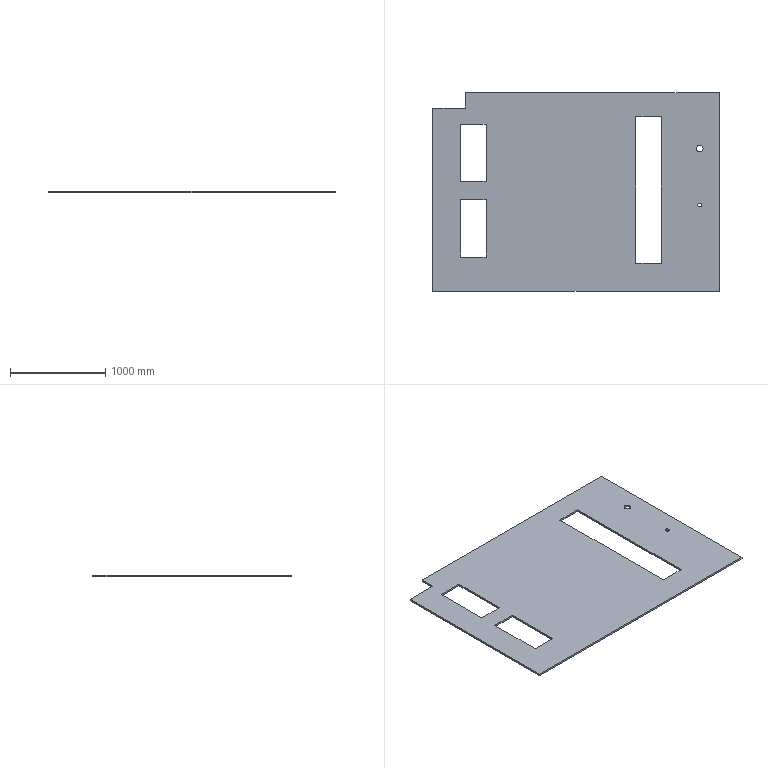Part | STEP file | 果蔬烘干机框架-104 | 1 solid | 24 faces | box 3000 x 2080 x 20 mm | volume 109217649 mm3 | plane 20 | cylinder 4 | commonest cylinder face diameters 40 x2 70 x2
STEP:
#1=CARTESIAN_POINT('',(1316.,-135.8,20.));
#2=VERTEX_POINT('',#1);
#3=CARTESIAN_POINT('',(1276.,-135.8,20.));
#4=VERTEX_POINT('',#3);
#5=CARTESIAN_POINT('',(1296.,-135.8,20.));
#6=DIRECTION('',(0.,0.,-1.));
#7=DIRECTION('',(-1.,0.,0.));
#8=AXIS2_PLACEMENT_3D('',#5,#6,#7);
#9=CIRCLE('',#8,20.);
#10=EDGE_CURVE('',#2,#4,#9,.T.);
#11=ORIENTED_EDGE('',*,*,#10,.F.);
#12=CARTESIAN_POINT('',(1316.,-135.8,0.));
#13=VERTEX_POINT('',#12);
#14=CARTESIAN_POINT('',(1316.,-135.8,20.));
#15=DIRECTION('',(0.,0.,-1.));
#16=VECTOR('',#15,1000.);
#17=LINE('',#14,#16);
#18=EDGE_CURVE('',#2,#13,#17,.T.);
#19=ORIENTED_EDGE('',*,*,#18,.T.);
#20=CARTESIAN_POINT('',(1276.,-135.8,0.));
#21=VERTEX_POINT('',#20);
#22=CARTESIAN_POINT('',(1296.,-135.8,0.));
#23=DIRECTION('',(0.,0.,-1.));
#24=DIRECTION('',(-1.,0.,0.));
#25=AXIS2_PLACEMENT_3D('',#22,#23,#24);
#26=CIRCLE('',#25,20.);
#27=EDGE_CURVE('',#13,#21,#26,.T.);
#28=ORIENTED_EDGE('',*,*,#27,.T.);
#29=CARTESIAN_POINT('',(1276.,-135.8,20.));
#30=DIRECTION('',(0.,0.,-1.));
#31=VECTOR('',#30,1000.);
#32=LINE('',#29,#31);
#33=EDGE_CURVE('',#4,#21,#32,.T.);
#34=ORIENTED_EDGE('',*,*,#33,.F.);
#35=EDGE_LOOP('',(#11,#19,#28,#34));
#36=FACE_OUTER_BOUND('',#35,.T.);
#37=CARTESIAN_POINT('',(1296.,-135.8,20.));
#38=DIRECTION('',(0.,0.,-1.));
#39=DIRECTION('',(-1.,0.,0.));
#40=AXIS2_PLACEMENT_3D('',#37,#38,#39);
#41=CYLINDRICAL_SURFACE('',#40,20.);
#42=ADVANCED_FACE('',(#36),#41,.F.);
#43=CARTESIAN_POINT('',(1331.,454.2,20.));
#44=VERTEX_POINT('',#43);
#45=CARTESIAN_POINT('',(1261.,454.2,20.));
#46=VERTEX_POINT('',#45);
#47=CARTESIAN_POINT('',(1296.,454.2,20.));
#48=DIRECTION('',(0.,0.,-1.));
#49=DIRECTION('',(-1.,0.,0.));
#50=AXIS2_PLACEMENT_3D('',#47,#48,#49);
#51=CIRCLE('',#50,35.);
#52=EDGE_CURVE('',#44,#46,#51,.T.);
#53=ORIENTED_EDGE('',*,*,#52,.F.);
#54=CARTESIAN_POINT('',(1331.,454.2,0.));
#55=VERTEX_POINT('',#54);
#56=CARTESIAN_POINT('',(1331.,454.2,20.));
#57=DIRECTION('',(0.,0.,-1.));
#58=VECTOR('',#57,1000.);
#59=LINE('',#56,#58);
#60=EDGE_CURVE('',#44,#55,#59,.T.);
#61=ORIENTED_EDGE('',*,*,#60,.T.);
#62=CARTESIAN_POINT('',(1261.,454.2,0.));
#63=VERTEX_POINT('',#62);
#64=CARTESIAN_POINT('',(1296.,454.2,0.));
#65=DIRECTION('',(0.,0.,-1.));
#66=DIRECTION('',(-1.,0.,0.));
#67=AXIS2_PLACEMENT_3D('',#64,#65,#66);
#68=CIRCLE('',#67,35.);
#69=EDGE_CURVE('',#55,#63,#68,.T.);
#70=ORIENTED_EDGE('',*,*,#69,.T.);
#71=CARTESIAN_POINT('',(1261.,454.2,20.));
#72=DIRECTION('',(0.,0.,-1.));
#73=VECTOR('',#72,1000.);
#74=LINE('',#71,#73);
#75=EDGE_CURVE('',#46,#63,#74,.T.);
#76=ORIENTED_EDGE('',*,*,#75,.F.);
#77=EDGE_LOOP('',(#53,#61,#70,#76));
#78=FACE_OUTER_BOUND('',#77,.T.);
#79=CARTESIAN_POINT('',(1296.,454.2,20.));
#80=DIRECTION('',(0.,0.,-1.));
#81=DIRECTION('',(-1.,0.,0.));
#82=AXIS2_PLACEMENT_3D('',#79,#80,#81);
#83=CYLINDRICAL_SURFACE('',#82,35.);
#84=ADVANCED_FACE('',(#78),#83,.F.);
#85=CARTESIAN_POINT('',(-1500.,880.,0.));
#86=VERTEX_POINT('',#85);
#87=CARTESIAN_POINT('',(-1500.,880.,20.));
#88=VERTEX_POINT('',#87);
#89=CARTESIAN_POINT('',(-1500.,880.,-80.));
#90=DIRECTION('',(0.,0.,1.));
#91=VECTOR('',#90,1000.);
#92=LINE('',#89,#91);
#93=EDGE_CURVE('',#86,#88,#92,.T.);
#94=ORIENTED_EDGE('',*,*,#93,.F.);
#95=CARTESIAN_POINT('',(-1500.,-1040.,0.));
#96=VERTEX_POINT('',#95);
#97=CARTESIAN_POINT('',(-1500.,1040.,0.));
#98=DIRECTION('',(0.,-1.,0.));
#99=VECTOR('',#98,1000.);
#100=LINE('',#97,#99);
#101=EDGE_CURVE('',#86,#96,#100,.T.);
#102=ORIENTED_EDGE('',*,*,#101,.T.);
#103=CARTESIAN_POINT('',(-1500.,-1040.,20.));
#104=VERTEX_POINT('',#103);
#105=CARTESIAN_POINT('',(-1500.,-1040.,20.));
#106=DIRECTION('',(0.,0.,-1.));
#107=VECTOR('',#106,1000.);
#108=LINE('',#105,#107);
#109=EDGE_CURVE('',#104,#96,#108,.T.);
#110=ORIENTED_EDGE('',*,*,#109,.F.);
#111=CARTESIAN_POINT('',(-1500.,1040.,20.));
#112=DIRECTION('',(0.,-1.,0.));
#113=VECTOR('',#112,1000.);
#114=LINE('',#111,#113);
#115=EDGE_CURVE('',#88,#104,#114,.T.);
#116=ORIENTED_EDGE('',*,*,#115,.F.);
#117=EDGE_LOOP('',(#94,#102,#110,#116));
#118=FACE_OUTER_BOUND('',#117,.T.);
#119=CARTESIAN_POINT('',(-1500.,1040.,20.));
#120=DIRECTION('',(1.,0.,0.));
#121=DIRECTION('',(0.,1.,0.));
#122=AXIS2_PLACEMENT_3D('',#119,#120,#121);
#123=PLANE('',#122);
#124=ADVANCED_FACE('',(#118),#123,.F.);
#125=CARTESIAN_POINT('',(1500.,-1040.,0.));
#126=VERTEX_POINT('',#125);
#127=CARTESIAN_POINT('',(1500.,1040.,0.));
#128=VERTEX_POINT('',#127);
#129=CARTESIAN_POINT('',(1500.,1040.,0.));
#130=DIRECTION('',(0.,1.,0.));
#131=VECTOR('',#130,1000.);
#132=LINE('',#129,#131);
#133=EDGE_CURVE('',#126,#128,#132,.T.);
#134=ORIENTED_EDGE('',*,*,#133,.T.);
#135=CARTESIAN_POINT('',(1500.,1040.,20.));
#136=VERTEX_POINT('',#135);
#137=CARTESIAN_POINT('',(1500.,1040.,20.));
#138=DIRECTION('',(0.,0.,-1.));
#139=VECTOR('',#138,1000.);
#140=LINE('',#137,#139);
#141=EDGE_CURVE('',#136,#128,#140,.T.);
#142=ORIENTED_EDGE('',*,*,#141,.F.);
#143=CARTESIAN_POINT('',(1500.,-1040.,20.));
#144=VERTEX_POINT('',#143);
#145=CARTESIAN_POINT('',(1500.,1040.,20.));
#146=DIRECTION('',(0.,1.,0.));
#147=VECTOR('',#146,1000.);
#148=LINE('',#145,#147);
#149=EDGE_CURVE('',#144,#136,#148,.T.);
#150=ORIENTED_EDGE('',*,*,#149,.F.);
#151=CARTESIAN_POINT('',(1500.,-1040.,20.));
#152=DIRECTION('',(0.,0.,-1.));
#153=VECTOR('',#152,1000.);
#154=LINE('',#151,#153);
#155=EDGE_CURVE('',#144,#126,#154,.T.);
#156=ORIENTED_EDGE('',*,*,#155,.T.);
#157=EDGE_LOOP('',(#134,#142,#150,#156));
#158=FACE_OUTER_BOUND('',#157,.T.);
#159=CARTESIAN_POINT('',(1500.,1040.,20.));
#160=DIRECTION('',(-1.,0.,0.));
#161=DIRECTION('',(0.,-1.,0.));
#162=AXIS2_PLACEMENT_3D('',#159,#160,#161);
#163=PLANE('',#162);
#164=ADVANCED_FACE('',(#158),#163,.F.);
#165=CARTESIAN_POINT('',(-1160.,1040.,0.));
#166=VERTEX_POINT('',#165);
#167=CARTESIAN_POINT('',(-1500.,1040.,0.));
#168=DIRECTION('',(-1.,0.,0.));
#169=VECTOR('',#168,1000.);
#170=LINE('',#167,#169);
#171=EDGE_CURVE('',#128,#166,#170,.T.);
#172=ORIENTED_EDGE('',*,*,#171,.T.);
#173=CARTESIAN_POINT('',(-1160.,1040.,20.));
#174=VERTEX_POINT('',#173);
#175=CARTESIAN_POINT('',(-1160.,1040.,-80.));
#176=DIRECTION('',(0.,0.,1.));
#177=VECTOR('',#176,1000.);
#178=LINE('',#175,#177);
#179=EDGE_CURVE('',#166,#174,#178,.T.);
#180=ORIENTED_EDGE('',*,*,#179,.T.);
#181=CARTESIAN_POINT('',(-1500.,1040.,20.));
#182=DIRECTION('',(-1.,0.,0.));
#183=VECTOR('',#182,1000.);
#184=LINE('',#181,#183);
#185=EDGE_CURVE('',#136,#174,#184,.T.);
#186=ORIENTED_EDGE('',*,*,#185,.F.);
#187=ORIENTED_EDGE('',*,*,#141,.T.);
#188=EDGE_LOOP('',(#172,#180,#186,#187));
#189=FACE_OUTER_BOUND('',#188,.T.);
#190=CARTESIAN_POINT('',(-1500.,1040.,20.));
#191=DIRECTION('',(0.,-1.,0.));
#192=DIRECTION('',(0.,0.,-1.));
#193=AXIS2_PLACEMENT_3D('',#190,#191,#192);
#194=PLANE('',#193);
#195=ADVANCED_FACE('',(#189),#194,.F.);
#196=CARTESIAN_POINT('',(-1500.,-1040.,0.));
#197=DIRECTION('',(1.,0.,0.));
#198=VECTOR('',#197,1000.);
#199=LINE('',#196,#198);
#200=EDGE_CURVE('',#96,#126,#199,.T.);
#201=ORIENTED_EDGE('',*,*,#200,.T.);
#202=ORIENTED_EDGE('',*,*,#155,.F.);
#203=CARTESIAN_POINT('',(-1500.,-1040.,20.));
#204=DIRECTION('',(1.,0.,0.));
#205=VECTOR('',#204,1000.);
#206=LINE('',#203,#205);
#207=EDGE_CURVE('',#104,#144,#206,.T.);
#208=ORIENTED_EDGE('',*,*,#207,.F.);
#209=ORIENTED_EDGE('',*,*,#109,.T.);
#210=EDGE_LOOP('',(#201,#202,#208,#209));
#211=FACE_OUTER_BOUND('',#210,.T.);
#212=CARTESIAN_POINT('',(-1500.,-1040.,20.));
#213=DIRECTION('',(0.,1.,0.));
#214=DIRECTION('',(0.,0.,1.));
#215=AXIS2_PLACEMENT_3D('',#212,#213,#214);
#216=PLANE('',#215);
#217=ADVANCED_FACE('',(#211),#216,.F.);
#218=CARTESIAN_POINT('',(1296.,-135.8,20.));
#219=DIRECTION('',(0.,0.,-1.));
#220=DIRECTION('',(-1.,0.,0.));
#221=AXIS2_PLACEMENT_3D('',#218,#219,#220);
#222=CIRCLE('',#221,20.);
#223=EDGE_CURVE('',#4,#2,#222,.T.);
#224=ORIENTED_EDGE('',*,*,#223,.T.);
#225=ORIENTED_EDGE('',*,*,#10,.T.);
#226=EDGE_LOOP('',(#224,#225));
#227=FACE_BOUND('',#226,.T.);
#228=CARTESIAN_POINT('',(1296.,454.2,20.));
#229=DIRECTION('',(0.,0.,-1.));
#230=DIRECTION('',(-1.,0.,0.));
#231=AXIS2_PLACEMENT_3D('',#228,#229,#230);
#232=CIRCLE('',#231,35.);
#233=EDGE_CURVE('',#46,#44,#232,.T.);
#234=ORIENTED_EDGE('',*,*,#233,.T.);
#235=ORIENTED_EDGE('',*,*,#52,.T.);
#236=EDGE_LOOP('',(#234,#235));
#237=FACE_BOUND('',#236,.T.);
#238=CARTESIAN_POINT('',(-943.,-81.276,20.));
#239=VERTEX_POINT('',#238);
#240=CARTESIAN_POINT('',(-943.,-681.324,20.));
#241=VERTEX_POINT('',#240);
#242=CARTESIAN_POINT('',(-943.,-81.276,20.));
#243=DIRECTION('',(0.,-1.,0.));
#244=VECTOR('',#243,1000.);
#245=LINE('',#242,#244);
#246=EDGE_CURVE('',#239,#241,#245,.T.);
#247=ORIENTED_EDGE('',*,*,#246,.T.);
#248=CARTESIAN_POINT('',(-1206.,-681.324,20.));
#249=VERTEX_POINT('',#248);
#250=CARTESIAN_POINT('',(-943.,-681.324,20.));
#251=DIRECTION('',(-1.,0.,0.));
#252=VECTOR('',#251,1000.);
#253=LINE('',#250,#252);
#254=EDGE_CURVE('',#241,#249,#253,.T.);
#255=ORIENTED_EDGE('',*,*,#254,.T.);
#256=CARTESIAN_POINT('',(-1206.,-81.276,20.));
#257=VERTEX_POINT('',#256);
#258=CARTESIAN_POINT('',(-1206.,-81.276,20.));
#259=DIRECTION('',(0.,1.,0.));
#260=VECTOR('',#259,1000.);
#261=LINE('',#258,#260);
#262=EDGE_CURVE('',#249,#257,#261,.T.);
#263=ORIENTED_EDGE('',*,*,#262,.T.);
#264=CARTESIAN_POINT('',(-943.,-81.276,20.));
#265=DIRECTION('',(1.,0.,0.));
#266=VECTOR('',#265,1000.);
#267=LINE('',#264,#266);
#268=EDGE_CURVE('',#257,#239,#267,.T.);
#269=ORIENTED_EDGE('',*,*,#268,.T.);
#270=EDGE_LOOP('',(#247,#255,#263,#269));
#271=FACE_BOUND('',#270,.T.);
#272=CARTESIAN_POINT('',(-943.,711.724,20.));
#273=VERTEX_POINT('',#272);
#274=CARTESIAN_POINT('',(-943.,111.676,20.));
#275=VERTEX_POINT('',#274);
#276=CARTESIAN_POINT('',(-943.,711.724,20.));
#277=DIRECTION('',(0.,-1.,0.));
#278=VECTOR('',#277,1000.);
#279=LINE('',#276,#278);
#280=EDGE_CURVE('',#273,#275,#279,.T.);
#281=ORIENTED_EDGE('',*,*,#280,.T.);
#282=CARTESIAN_POINT('',(-1206.,111.676,20.));
#283=VERTEX_POINT('',#282);
#284=CARTESIAN_POINT('',(-943.,111.676,20.));
#285=DIRECTION('',(-1.,0.,0.));
#286=VECTOR('',#285,1000.);
#287=LINE('',#284,#286);
#288=EDGE_CURVE('',#275,#283,#287,.T.);
#289=ORIENTED_EDGE('',*,*,#288,.T.);
#290=CARTESIAN_POINT('',(-1206.,711.724,20.));
#291=VERTEX_POINT('',#290);
#292=CARTESIAN_POINT('',(-1206.,711.724,20.));
#293=DIRECTION('',(0.,1.,0.));
#294=VECTOR('',#293,1000.);
#295=LINE('',#292,#294);
#296=EDGE_CURVE('',#283,#291,#295,.T.);
#297=ORIENTED_EDGE('',*,*,#296,.T.);
#298=CARTESIAN_POINT('',(-943.,711.724,20.));
#299=DIRECTION('',(1.,0.,0.));
#300=VECTOR('',#299,1000.);
#301=LINE('',#298,#300);
#302=EDGE_CURVE('',#291,#273,#301,.T.);
#303=ORIENTED_EDGE('',*,*,#302,.T.);
#304=EDGE_LOOP('',(#281,#289,#297,#303));
#305=FACE_BOUND('',#304,.T.);
#306=CARTESIAN_POINT('',(891.55,788.541,20.));
#307=VERTEX_POINT('',#306);
#308=CARTESIAN_POINT('',(891.55,-746.951,20.));
#309=VERTEX_POINT('',#308);
#310=CARTESIAN_POINT('',(891.55,788.541,20.));
#311=DIRECTION('',(0.,-1.,0.));
#312=VECTOR('',#311,1000.);
#313=LINE('',#310,#312);
#314=EDGE_CURVE('',#307,#309,#313,.T.);
#315=ORIENTED_EDGE('',*,*,#314,.T.);
#316=CARTESIAN_POINT('',(628.45,-746.951,20.));
#317=VERTEX_POINT('',#316);
#318=CARTESIAN_POINT('',(891.55,-746.951,20.));
#319=DIRECTION('',(-1.,0.,0.));
#320=VECTOR('',#319,1000.);
#321=LINE('',#318,#320);
#322=EDGE_CURVE('',#309,#317,#321,.T.);
#323=ORIENTED_EDGE('',*,*,#322,.T.);
#324=CARTESIAN_POINT('',(628.45,788.541,20.));
#325=VERTEX_POINT('',#324);
#326=CARTESIAN_POINT('',(628.45,788.541,20.));
#327=DIRECTION('',(0.,1.,0.));
#328=VECTOR('',#327,1000.);
#329=LINE('',#326,#328);
#330=EDGE_CURVE('',#317,#325,#329,.T.);
#331=ORIENTED_EDGE('',*,*,#330,.T.);
#332=CARTESIAN_POINT('',(891.55,788.541,20.));
#333=DIRECTION('',(1.,0.,0.));
#334=VECTOR('',#333,1000.);
#335=LINE('',#332,#334);
#336=EDGE_CURVE('',#325,#307,#335,.T.);
#337=ORIENTED_EDGE('',*,*,#336,.T.);
#338=EDGE_LOOP('',(#315,#323,#331,#337));
#339=FACE_BOUND('',#338,.T.);
#340=CARTESIAN_POINT('',(-1160.,880.,20.));
#341=VERTEX_POINT('',#340);
#342=CARTESIAN_POINT('',(-1500.,880.,20.));
#343=DIRECTION('',(1.,0.,0.));
#344=VECTOR('',#343,1000.);
#345=LINE('',#342,#344);
#346=EDGE_CURVE('',#88,#341,#345,.T.);
#347=ORIENTED_EDGE('',*,*,#346,.F.);
#348=ORIENTED_EDGE('',*,*,#115,.T.);
#349=ORIENTED_EDGE('',*,*,#207,.T.);
#350=ORIENTED_EDGE('',*,*,#149,.T.);
#351=ORIENTED_EDGE('',*,*,#185,.T.);
#352=CARTESIAN_POINT('',(-1160.,1040.,20.));
#353=DIRECTION('',(0.,1.,0.));
#354=VECTOR('',#353,1000.);
#355=LINE('',#352,#354);
#356=EDGE_CURVE('',#341,#174,#355,.T.);
#357=ORIENTED_EDGE('',*,*,#356,.F.);
#358=EDGE_LOOP('',(#347,#348,#349,#350,#351,#357));
#359=FACE_OUTER_BOUND('',#358,.T.);
#360=CARTESIAN_POINT('',(0.,0.,20.));
#361=DIRECTION('',(0.,0.,1.));
#362=DIRECTION('',(1.,0.,0.));
#363=AXIS2_PLACEMENT_3D('',#360,#361,#362);
#364=PLANE('',#363);
#365=ADVANCED_FACE('',(#227,#237,#271,#305,#339,#359),#364,.T.);
#366=CARTESIAN_POINT('',(1296.,-135.8,0.));
#367=DIRECTION('',(0.,0.,-1.));
#368=DIRECTION('',(-1.,0.,0.));
#369=AXIS2_PLACEMENT_3D('',#366,#367,#368);
#370=CIRCLE('',#369,20.);
#371=EDGE_CURVE('',#21,#13,#370,.T.);
#372=ORIENTED_EDGE('',*,*,#371,.F.);
#373=ORIENTED_EDGE('',*,*,#27,.F.);
#374=EDGE_LOOP('',(#372,#373));
#375=FACE_BOUND('',#374,.T.);
#376=CARTESIAN_POINT('',(1296.,454.2,0.));
#377=DIRECTION('',(0.,0.,-1.));
#378=DIRECTION('',(-1.,0.,0.));
#379=AXIS2_PLACEMENT_3D('',#376,#377,#378);
#380=CIRCLE('',#379,35.);
#381=EDGE_CURVE('',#63,#55,#380,.T.);
#382=ORIENTED_EDGE('',*,*,#381,.F.);
#383=ORIENTED_EDGE('',*,*,#69,.F.);
#384=EDGE_LOOP('',(#382,#383));
#385=FACE_BOUND('',#384,.T.);
#386=CARTESIAN_POINT('',(-943.,-681.324,0.));
#387=VERTEX_POINT('',#386);
#388=CARTESIAN_POINT('',(-1206.,-681.324,0.));
#389=VERTEX_POINT('',#388);
#390=CARTESIAN_POINT('',(-943.,-681.324,0.));
#391=DIRECTION('',(-1.,0.,0.));
#392=VECTOR('',#391,1000.);
#393=LINE('',#390,#392);
#394=EDGE_CURVE('',#387,#389,#393,.T.);
#395=ORIENTED_EDGE('',*,*,#394,.F.);
#396=CARTESIAN_POINT('',(-943.,-81.276,0.));
#397=VERTEX_POINT('',#396);
#398=CARTESIAN_POINT('',(-943.,-81.276,0.));
#399=DIRECTION('',(0.,-1.,0.));
#400=VECTOR('',#399,1000.);
#401=LINE('',#398,#400);
#402=EDGE_CURVE('',#397,#387,#401,.T.);
#403=ORIENTED_EDGE('',*,*,#402,.F.);
#404=CARTESIAN_POINT('',(-1206.,-81.276,0.));
#405=VERTEX_POINT('',#404);
#406=CARTESIAN_POINT('',(-943.,-81.276,0.));
#407=DIRECTION('',(1.,0.,0.));
#408=VECTOR('',#407,1000.);
#409=LINE('',#406,#408);
#410=EDGE_CURVE('',#405,#397,#409,.T.);
#411=ORIENTED_EDGE('',*,*,#410,.F.);
#412=CARTESIAN_POINT('',(-1206.,-81.276,0.));
#413=DIRECTION('',(0.,1.,0.));
#414=VECTOR('',#413,1000.);
#415=LINE('',#412,#414);
#416=EDGE_CURVE('',#389,#405,#415,.T.);
#417=ORIENTED_EDGE('',*,*,#416,.F.);
#418=EDGE_LOOP('',(#395,#403,#411,#417));
#419=FACE_BOUND('',#418,.T.);
#420=CARTESIAN_POINT('',(-943.,111.676,0.));
#421=VERTEX_POINT('',#420);
#422=CARTESIAN_POINT('',(-1206.,111.676,0.));
#423=VERTEX_POINT('',#422);
#424=CARTESIAN_POINT('',(-943.,111.676,0.));
#425=DIRECTION('',(-1.,0.,0.));
#426=VECTOR('',#425,1000.);
#427=LINE('',#424,#426);
#428=EDGE_CURVE('',#421,#423,#427,.T.);
#429=ORIENTED_EDGE('',*,*,#428,.F.);
#430=CARTESIAN_POINT('',(-943.,711.724,0.));
#431=VERTEX_POINT('',#430);
#432=CARTESIAN_POINT('',(-943.,711.724,0.));
#433=DIRECTION('',(0.,-1.,0.));
#434=VECTOR('',#433,1000.);
#435=LINE('',#432,#434);
#436=EDGE_CURVE('',#431,#421,#435,.T.);
#437=ORIENTED_EDGE('',*,*,#436,.F.);
#438=CARTESIAN_POINT('',(-1206.,711.724,0.));
#439=VERTEX_POINT('',#438);
#440=CARTESIAN_POINT('',(-943.,711.724,0.));
#441=DIRECTION('',(1.,0.,0.));
#442=VECTOR('',#441,1000.);
#443=LINE('',#440,#442);
#444=EDGE_CURVE('',#439,#431,#443,.T.);
#445=ORIENTED_EDGE('',*,*,#444,.F.);
#446=CARTESIAN_POINT('',(-1206.,711.724,0.));
#447=DIRECTION('',(0.,1.,0.));
#448=VECTOR('',#447,1000.);
#449=LINE('',#446,#448);
#450=EDGE_CURVE('',#423,#439,#449,.T.);
#451=ORIENTED_EDGE('',*,*,#450,.F.);
#452=EDGE_LOOP('',(#429,#437,#445,#451));
#453=FACE_BOUND('',#452,.T.);
#454=CARTESIAN_POINT('',(891.55,-746.951,0.));
#455=VERTEX_POINT('',#454);
#456=CARTESIAN_POINT('',(628.45,-746.951,0.));
#457=VERTEX_POINT('',#456);
#458=CARTESIAN_POINT('',(891.55,-746.951,0.));
#459=DIRECTION('',(-1.,0.,0.));
#460=VECTOR('',#459,1000.);
#461=LINE('',#458,#460);
#462=EDGE_CURVE('',#455,#457,#461,.T.);
#463=ORIENTED_EDGE('',*,*,#462,.F.);
#464=CARTESIAN_POINT('',(891.55,788.541,0.));
#465=VERTEX_POINT('',#464);
#466=CARTESIAN_POINT('',(891.55,788.541,0.));
#467=DIRECTION('',(0.,-1.,0.));
#468=VECTOR('',#467,1000.);
#469=LINE('',#466,#468);
#470=EDGE_CURVE('',#465,#455,#469,.T.);
#471=ORIENTED_EDGE('',*,*,#470,.F.);
#472=CARTESIAN_POINT('',(628.45,788.541,0.));
#473=VERTEX_POINT('',#472);
#474=CARTESIAN_POINT('',(891.55,788.541,0.));
#475=DIRECTION('',(1.,0.,0.));
#476=VECTOR('',#475,1000.);
#477=LINE('',#474,#476);
#478=EDGE_CURVE('',#473,#465,#477,.T.);
#479=ORIENTED_EDGE('',*,*,#478,.F.);
#480=CARTESIAN_POINT('',(628.45,788.541,0.));
#481=DIRECTION('',(0.,1.,0.));
#482=VECTOR('',#481,1000.);
#483=LINE('',#480,#482);
#484=EDGE_CURVE('',#457,#473,#483,.T.);
#485=ORIENTED_EDGE('',*,*,#484,.F.);
#486=EDGE_LOOP('',(#463,#471,#479,#485));
#487=FACE_BOUND('',#486,.T.);
#488=CARTESIAN_POINT('',(-1160.,880.,0.));
#489=VERTEX_POINT('',#488);
#490=CARTESIAN_POINT('',(0.,880.,0.));
#491=DIRECTION('',(1.,0.,0.));
#492=VECTOR('',#491,1000.);
#493=LINE('',#490,#492);
#494=EDGE_CURVE('',#86,#489,#493,.T.);
#495=ORIENTED_EDGE('',*,*,#494,.T.);
#496=CARTESIAN_POINT('',(-1160.,0.,0.));
#497=DIRECTION('',(0.,1.,0.));
#498=VECTOR('',#497,1000.);
#499=LINE('',#496,#498);
#500=EDGE_CURVE('',#489,#166,#499,.T.);
#501=ORIENTED_EDGE('',*,*,#500,.T.);
#502=ORIENTED_EDGE('',*,*,#171,.F.);
#503=ORIENTED_EDGE('',*,*,#133,.F.);
#504=ORIENTED_EDGE('',*,*,#200,.F.);
#505=ORIENTED_EDGE('',*,*,#101,.F.);
#506=EDGE_LOOP('',(#495,#501,#502,#503,#504,#505));
#507=FACE_OUTER_BOUND('',#506,.T.);
#508=CARTESIAN_POINT('',(0.,0.,0.));
#509=DIRECTION('',(0.,0.,1.));
#510=DIRECTION('',(1.,0.,0.));
#511=AXIS2_PLACEMENT_3D('',#508,#509,#510);
#512=PLANE('',#511);
#513=ADVANCED_FACE('',(#375,#385,#419,#453,#487,#507),#512,.F.);
#514=CARTESIAN_POINT('',(-1160.,880.,-80.));
#515=DIRECTION('',(0.,0.,1.));
#516=VECTOR('',#515,1000.);
#517=LINE('',#514,#516);
#518=EDGE_CURVE('',#489,#341,#517,.T.);
#519=ORIENTED_EDGE('',*,*,#518,.T.);
#520=ORIENTED_EDGE('',*,*,#356,.T.);
#521=ORIENTED_EDGE('',*,*,#179,.F.);
#522=ORIENTED_EDGE('',*,*,#500,.F.);
#523=EDGE_LOOP('',(#519,#520,#521,#522));
#524=FACE_OUTER_BOUND('',#523,.T.);
#525=CARTESIAN_POINT('',(-1160.,1040.,-80.));
#526=DIRECTION('',(1.,0.,0.));
#527=DIRECTION('',(0.,0.,-1.));
#528=AXIS2_PLACEMENT_3D('',#525,#526,#527);
#529=PLANE('',#528);
#530=ADVANCED_FACE('',(#524),#529,.F.);
#531=ORIENTED_EDGE('',*,*,#93,.T.);
#532=ORIENTED_EDGE('',*,*,#346,.T.);
#533=ORIENTED_EDGE('',*,*,#518,.F.);
#534=ORIENTED_EDGE('',*,*,#494,.F.);
#535=EDGE_LOOP('',(#531,#532,#533,#534));
#536=FACE_OUTER_BOUND('',#535,.T.);
#537=CARTESIAN_POINT('',(-1500.,880.,-80.));
#538=DIRECTION('',(0.,-1.,0.));
#539=DIRECTION('',(0.,0.,-1.));
#540=AXIS2_PLACEMENT_3D('',#537,#538,#539);
#541=PLANE('',#540);
#542=ADVANCED_FACE('',(#536),#541,.F.);
#543=ORIENTED_EDGE('',*,*,#470,.T.);
#544=CARTESIAN_POINT('',(891.55,-746.951,20.));
#545=DIRECTION('',(0.,0.,-1.));
#546=VECTOR('',#545,1000.);
#547=LINE('',#544,#546);
#548=EDGE_CURVE('',#309,#455,#547,.T.);
#549=ORIENTED_EDGE('',*,*,#548,.F.);
#550=ORIENTED_EDGE('',*,*,#314,.F.);
#551=CARTESIAN_POINT('',(891.55,788.541,20.));
#552=DIRECTION('',(0.,0.,-1.));
#553=VECTOR('',#552,1000.);
#554=LINE('',#551,#553);
#555=EDGE_CURVE('',#307,#465,#554,.T.);
#556=ORIENTED_EDGE('',*,*,#555,.T.);
#557=EDGE_LOOP('',(#543,#549,#550,#556));
#558=FACE_OUTER_BOUND('',#557,.T.);
#559=CARTESIAN_POINT('',(891.55,788.541,20.));
#560=DIRECTION('',(1.,0.,0.));
#561=DIRECTION('',(0.,1.,0.));
#562=AXIS2_PLACEMENT_3D('',#559,#560,#561);
#563=PLANE('',#562);
#564=ADVANCED_FACE('',(#558),#563,.F.);
#565=ORIENTED_EDGE('',*,*,#478,.T.);
#566=ORIENTED_EDGE('',*,*,#555,.F.);
#567=ORIENTED_EDGE('',*,*,#336,.F.);
#568=CARTESIAN_POINT('',(628.45,788.541,20.));
#569=DIRECTION('',(0.,0.,-1.));
#570=VECTOR('',#569,1000.);
#571=LINE('',#568,#570);
#572=EDGE_CURVE('',#325,#473,#571,.T.);
#573=ORIENTED_EDGE('',*,*,#572,.T.);
#574=EDGE_LOOP('',(#565,#566,#567,#573));
#575=FACE_OUTER_BOUND('',#574,.T.);
#576=CARTESIAN_POINT('',(891.55,788.541,20.));
#577=DIRECTION('',(0.,1.,0.));
#578=DIRECTION('',(0.,0.,1.));
#579=AXIS2_PLACEMENT_3D('',#576,#577,#578);
#580=PLANE('',#579);
#581=ADVANCED_FACE('',(#575),#580,.F.);
#582=ORIENTED_EDGE('',*,*,#484,.T.);
#583=ORIENTED_EDGE('',*,*,#572,.F.);
#584=ORIENTED_EDGE('',*,*,#330,.F.);
#585=CARTESIAN_POINT('',(628.45,-746.951,20.));
#586=DIRECTION('',(0.,0.,-1.));
#587=VECTOR('',#586,1000.);
#588=LINE('',#585,#587);
#589=EDGE_CURVE('',#317,#457,#588,.T.);
#590=ORIENTED_EDGE('',*,*,#589,.T.);
#591=EDGE_LOOP('',(#582,#583,#584,#590));
#592=FACE_OUTER_BOUND('',#591,.T.);
#593=CARTESIAN_POINT('',(628.45,788.541,20.));
#594=DIRECTION('',(-1.,0.,0.));
#595=DIRECTION('',(0.,-1.,0.));
#596=AXIS2_PLACEMENT_3D('',#593,#594,#595);
#597=PLANE('',#596);
#598=ADVANCED_FACE('',(#592),#597,.F.);
#599=ORIENTED_EDGE('',*,*,#462,.T.);
#600=ORIENTED_EDGE('',*,*,#589,.F.);
#601=ORIENTED_EDGE('',*,*,#322,.F.);
#602=ORIENTED_EDGE('',*,*,#548,.T.);
#603=EDGE_LOOP('',(#599,#600,#601,#602));
#604=FACE_OUTER_BOUND('',#603,.T.);
#605=CARTESIAN_POINT('',(891.55,-746.951,20.));
#606=DIRECTION('',(0.,-1.,0.));
#607=DIRECTION('',(0.,0.,-1.));
#608=AXIS2_PLACEMENT_3D('',#605,#606,#607);
#609=PLANE('',#608);
#610=ADVANCED_FACE('',(#604),#609,.F.);
#611=ORIENTED_EDGE('',*,*,#436,.T.);
#612=CARTESIAN_POINT('',(-943.,111.676,20.));
#613=DIRECTION('',(0.,0.,-1.));
#614=VECTOR('',#613,1000.);
#615=LINE('',#612,#614);
#616=EDGE_CURVE('',#275,#421,#615,.T.);
#617=ORIENTED_EDGE('',*,*,#616,.F.);
#618=ORIENTED_EDGE('',*,*,#280,.F.);
#619=CARTESIAN_POINT('',(-943.,711.724,20.));
#620=DIRECTION('',(0.,0.,-1.));
#621=VECTOR('',#620,1000.);
#622=LINE('',#619,#621);
#623=EDGE_CURVE('',#273,#431,#622,.T.);
#624=ORIENTED_EDGE('',*,*,#623,.T.);
#625=EDGE_LOOP('',(#611,#617,#618,#624));
#626=FACE_OUTER_BOUND('',#625,.T.);
#627=CARTESIAN_POINT('',(-943.,711.724,20.));
#628=DIRECTION('',(1.,0.,0.));
#629=DIRECTION('',(0.,1.,0.));
#630=AXIS2_PLACEMENT_3D('',#627,#628,#629);
#631=PLANE('',#630);
#632=ADVANCED_FACE('',(#626),#631,.F.);
#633=ORIENTED_EDGE('',*,*,#444,.T.);
#634=ORIENTED_EDGE('',*,*,#623,.F.);
#635=ORIENTED_EDGE('',*,*,#302,.F.);
#636=CARTESIAN_POINT('',(-1206.,711.724,20.));
#637=DIRECTION('',(0.,0.,-1.));
#638=VECTOR('',#637,1000.);
#639=LINE('',#636,#638);
#640=EDGE_CURVE('',#291,#439,#639,.T.);
#641=ORIENTED_EDGE('',*,*,#640,.T.);
#642=EDGE_LOOP('',(#633,#634,#635,#641));
#643=FACE_OUTER_BOUND('',#642,.T.);
#644=CARTESIAN_POINT('',(-943.,711.724,20.));
#645=DIRECTION('',(0.,1.,0.));
#646=DIRECTION('',(0.,0.,1.));
#647=AXIS2_PLACEMENT_3D('',#644,#645,#646);
#648=PLANE('',#647);
#649=ADVANCED_FACE('',(#643),#648,.F.);
#650=ORIENTED_EDGE('',*,*,#450,.T.);
#651=ORIENTED_EDGE('',*,*,#640,.F.);
#652=ORIENTED_EDGE('',*,*,#296,.F.);
#653=CARTESIAN_POINT('',(-1206.,111.676,20.));
#654=DIRECTION('',(0.,0.,-1.));
#655=VECTOR('',#654,1000.);
#656=LINE('',#653,#655);
#657=EDGE_CURVE('',#283,#423,#656,.T.);
#658=ORIENTED_EDGE('',*,*,#657,.T.);
#659=EDGE_LOOP('',(#650,#651,#652,#658));
#660=FACE_OUTER_BOUND('',#659,.T.);
#661=CARTESIAN_POINT('',(-1206.,711.724,20.));
#662=DIRECTION('',(-1.,0.,0.));
#663=DIRECTION('',(0.,0.,1.));
#664=AXIS2_PLACEMENT_3D('',#661,#662,#663);
#665=PLANE('',#664);
#666=ADVANCED_FACE('',(#660),#665,.F.);
#667=ORIENTED_EDGE('',*,*,#428,.T.);
#668=ORIENTED_EDGE('',*,*,#657,.F.);
#669=ORIENTED_EDGE('',*,*,#288,.F.);
#670=ORIENTED_EDGE('',*,*,#616,.T.);
#671=EDGE_LOOP('',(#667,#668,#669,#670));
#672=FACE_OUTER_BOUND('',#671,.T.);
#673=CARTESIAN_POINT('',(-943.,111.676,20.));
#674=DIRECTION('',(0.,-1.,0.));
#675=DIRECTION('',(0.,0.,-1.));
#676=AXIS2_PLACEMENT_3D('',#673,#674,#675);
#677=PLANE('',#676);
#678=ADVANCED_FACE('',(#672),#677,.F.);
#679=ORIENTED_EDGE('',*,*,#402,.T.);
#680=CARTESIAN_POINT('',(-943.,-681.324,20.));
#681=DIRECTION('',(0.,0.,-1.));
#682=VECTOR('',#681,1000.);
#683=LINE('',#680,#682);
#684=EDGE_CURVE('',#241,#387,#683,.T.);
#685=ORIENTED_EDGE('',*,*,#684,.F.);
#686=ORIENTED_EDGE('',*,*,#246,.F.);
#687=CARTESIAN_POINT('',(-943.,-81.276,20.));
#688=DIRECTION('',(0.,0.,-1.));
#689=VECTOR('',#688,1000.);
#690=LINE('',#687,#689);
#691=EDGE_CURVE('',#239,#397,#690,.T.);
#692=ORIENTED_EDGE('',*,*,#691,.T.);
#693=EDGE_LOOP('',(#679,#685,#686,#692));
#694=FACE_OUTER_BOUND('',#693,.T.);
#695=CARTESIAN_POINT('',(-943.,-81.276,20.));
#696=DIRECTION('',(1.,0.,0.));
#697=DIRECTION('',(0.,1.,0.));
#698=AXIS2_PLACEMENT_3D('',#695,#696,#697);
#699=PLANE('',#698);
#700=ADVANCED_FACE('',(#694),#699,.F.);
#701=ORIENTED_EDGE('',*,*,#410,.T.);
#702=ORIENTED_EDGE('',*,*,#691,.F.);
#703=ORIENTED_EDGE('',*,*,#268,.F.);
#704=CARTESIAN_POINT('',(-1206.,-81.276,20.));
#705=DIRECTION('',(0.,0.,-1.));
#706=VECTOR('',#705,1000.);
#707=LINE('',#704,#706);
#708=EDGE_CURVE('',#257,#405,#707,.T.);
#709=ORIENTED_EDGE('',*,*,#708,.T.);
#710=EDGE_LOOP('',(#701,#702,#703,#709));
#711=FACE_OUTER_BOUND('',#710,.T.);
#712=CARTESIAN_POINT('',(-943.,-81.276,20.));
#713=DIRECTION('',(0.,1.,0.));
#714=DIRECTION('',(0.,0.,1.));
#715=AXIS2_PLACEMENT_3D('',#712,#713,#714);
#716=PLANE('',#715);
#717=ADVANCED_FACE('',(#711),#716,.F.);
#718=ORIENTED_EDGE('',*,*,#416,.T.);
#719=ORIENTED_EDGE('',*,*,#708,.F.);
#720=ORIENTED_EDGE('',*,*,#262,.F.);
#721=CARTESIAN_POINT('',(-1206.,-681.324,20.));
#722=DIRECTION('',(0.,0.,-1.));
#723=VECTOR('',#722,1000.);
#724=LINE('',#721,#723);
#725=EDGE_CURVE('',#249,#389,#724,.T.);
#726=ORIENTED_EDGE('',*,*,#725,.T.);
#727=EDGE_LOOP('',(#718,#719,#720,#726));
#728=FACE_OUTER_BOUND('',#727,.T.);
#729=CARTESIAN_POINT('',(-1206.,-81.276,20.));
#730=DIRECTION('',(-1.,0.,0.));
#731=DIRECTION('',(0.,0.,1.));
#732=AXIS2_PLACEMENT_3D('',#729,#730,#731);
#733=PLANE('',#732);
#734=ADVANCED_FACE('',(#728),#733,.F.);
#735=ORIENTED_EDGE('',*,*,#394,.T.);
#736=ORIENTED_EDGE('',*,*,#725,.F.);
#737=ORIENTED_EDGE('',*,*,#254,.F.);
#738=ORIENTED_EDGE('',*,*,#684,.T.);
#739=EDGE_LOOP('',(#735,#736,#737,#738));
#740=FACE_OUTER_BOUND('',#739,.T.);
#741=CARTESIAN_POINT('',(-943.,-681.324,20.));
#742=DIRECTION('',(0.,-1.,0.));
#743=DIRECTION('',(0.,0.,-1.));
#744=AXIS2_PLACEMENT_3D('',#741,#742,#743);
#745=PLANE('',#744);
#746=ADVANCED_FACE('',(#740),#745,.F.);
#747=ORIENTED_EDGE('',*,*,#60,.F.);
#748=ORIENTED_EDGE('',*,*,#233,.F.);
#749=ORIENTED_EDGE('',*,*,#75,.T.);
#750=ORIENTED_EDGE('',*,*,#381,.T.);
#751=EDGE_LOOP('',(#747,#748,#749,#750));
#752=FACE_OUTER_BOUND('',#751,.T.);
#753=CARTESIAN_POINT('',(1296.,454.2,20.));
#754=DIRECTION('',(0.,0.,-1.));
#755=DIRECTION('',(-1.,0.,0.));
#756=AXIS2_PLACEMENT_3D('',#753,#754,#755);
#757=CYLINDRICAL_SURFACE('',#756,35.);
#758=ADVANCED_FACE('',(#752),#757,.F.);
#759=ORIENTED_EDGE('',*,*,#18,.F.);
#760=ORIENTED_EDGE('',*,*,#223,.F.);
#761=ORIENTED_EDGE('',*,*,#33,.T.);
#762=ORIENTED_EDGE('',*,*,#371,.T.);
#763=EDGE_LOOP('',(#759,#760,#761,#762));
#764=FACE_OUTER_BOUND('',#763,.T.);
#765=CARTESIAN_POINT('',(1296.,-135.8,20.));
#766=DIRECTION('',(0.,0.,-1.));
#767=DIRECTION('',(-1.,0.,0.));
#768=AXIS2_PLACEMENT_3D('',#765,#766,#767);
#769=CYLINDRICAL_SURFACE('',#768,20.);
#770=ADVANCED_FACE('',(#764),#769,.F.);
#771=CLOSED_SHELL('',(#42,#84,#124,#164,#195,#217,#365,#513,#530,#542,#564,#581,#598,#610,#632,#649,#666,#678,#700,#717,#734,#746,#758,#770));
#772=MANIFOLD_SOLID_BREP('',#771);
#773=CARTESIAN_POINT('',(0.,0.,0.));
#774=DIRECTION('',(0.,0.,1.));
#775=DIRECTION('',(1.,0.,0.));
#776=AXIS2_PLACEMENT_3D('',#773,#774,#775);
#777=(LENGTH_UNIT()NAMED_UNIT(*)SI_UNIT(.MILLI.,.METRE.));
#778=UNCERTAINTY_MEASURE_WITH_UNIT(LENGTH_MEASURE(0.00001),#777,'','');
#779=(NAMED_UNIT(*)PLANE_ANGLE_UNIT()SI_UNIT($,.RADIAN.));
#780=(NAMED_UNIT(*)SI_UNIT($,.STERADIAN.)SOLID_ANGLE_UNIT());
#781=(GEOMETRIC_REPRESENTATION_CONTEXT(3)GLOBAL_UNCERTAINTY_ASSIGNED_CONTEXT((#778))GLOBAL_UNIT_ASSIGNED_CONTEXT((#777,#779,#780))REPRESENTATION_CONTEXT('',''));
#782=ADVANCED_BREP_SHAPE_REPRESENTATION('',(#772,#776),#781);